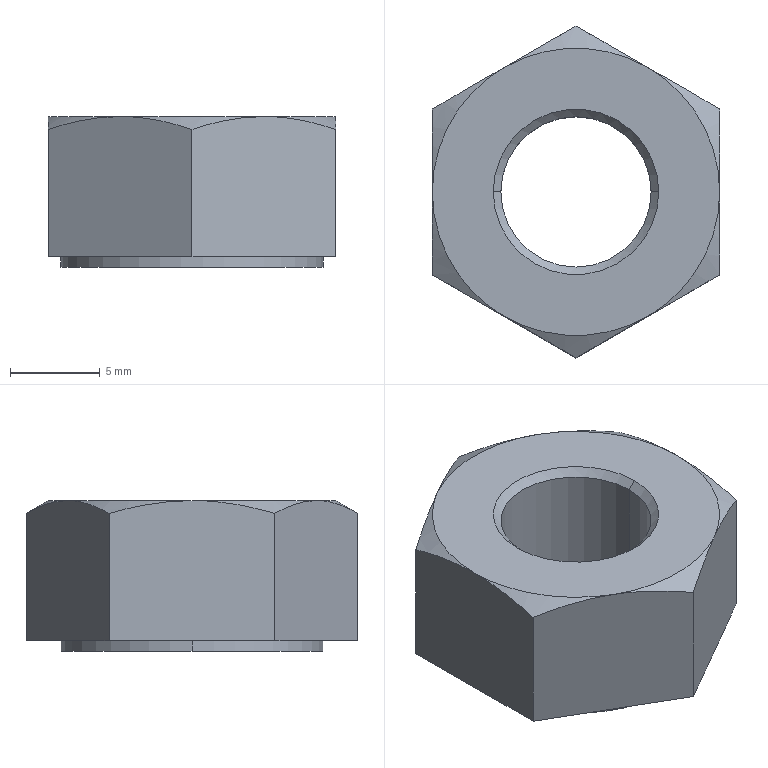Part | SolidWorks | features Cut 2, Chamfer 1, Extrusion 1 | 1 solid | 23 faces | box 16 x 18.475 x 8.4 mm | volume 1358 mm3 | cone 10 | plane 9 | cylinder 4 | commonest cylinder face diameters 8.376 x2 14.6 x2
STEP:
#1=CARTESIAN_POINT('',(-4.188,0.,7.98));
#2=VERTEX_POINT('',#1);
#3=CARTESIAN_POINT('',(4.188,0.,7.98));
#4=VERTEX_POINT('',#3);
#5=CARTESIAN_POINT('',(0.,0.,7.98));
#6=DIRECTION('',(0.,0.,1.));
#7=DIRECTION('',(1.,0.,0.));
#8=AXIS2_PLACEMENT_3D('',#5,#6,#7);
#9=CIRCLE('',#8,4.188);
#10=EDGE_CURVE('',#2,#4,#9,.T.);
#11=ORIENTED_EDGE('',*,*,#10,.F.);
#12=CARTESIAN_POINT('',(-4.608,0.,8.4));
#13=VERTEX_POINT('',#12);
#14=CARTESIAN_POINT('',(-4.188,0.,7.98));
#15=DIRECTION('',(-0.7071,0.,0.7071));
#16=VECTOR('',#15,1000.);
#17=LINE('',#14,#16);
#18=EDGE_CURVE('',#2,#13,#17,.T.);
#19=ORIENTED_EDGE('',*,*,#18,.T.);
#20=CARTESIAN_POINT('',(4.608,0.,8.4));
#21=VERTEX_POINT('',#20);
#22=CARTESIAN_POINT('',(0.,0.,8.4));
#23=DIRECTION('',(0.,0.,-1.));
#24=DIRECTION('',(1.,0.,0.));
#25=AXIS2_PLACEMENT_3D('',#22,#23,#24);
#26=CIRCLE('',#25,4.608);
#27=EDGE_CURVE('',#21,#13,#26,.T.);
#28=ORIENTED_EDGE('',*,*,#27,.F.);
#29=CARTESIAN_POINT('',(4.188,0.,7.98));
#30=DIRECTION('',(0.7071,0.,0.7071));
#31=VECTOR('',#30,1000.);
#32=LINE('',#29,#31);
#33=EDGE_CURVE('',#4,#21,#32,.T.);
#34=ORIENTED_EDGE('',*,*,#33,.F.);
#35=EDGE_LOOP('',(#11,#19,#28,#34));
#36=FACE_OUTER_BOUND('',#35,.T.);
#37=CARTESIAN_POINT('',(0.,0.,7.98));
#38=DIRECTION('',(0.,0.,1.));
#39=DIRECTION('',(1.,0.,0.));
#40=AXIS2_PLACEMENT_3D('',#37,#38,#39);
#41=CONICAL_SURFACE('',#40,4.188,0.7854);
#42=ADVANCED_FACE('',(#36),#41,.F.);
#43=CARTESIAN_POINT('',(4.188,0.,0.42));
#44=VERTEX_POINT('',#43);
#45=CARTESIAN_POINT('',(-4.188,0.,0.42));
#46=VERTEX_POINT('',#45);
#47=CARTESIAN_POINT('',(0.,0.,0.42));
#48=DIRECTION('',(0.,0.,-1.));
#49=DIRECTION('',(1.,0.,0.));
#50=AXIS2_PLACEMENT_3D('',#47,#48,#49);
#51=CIRCLE('',#50,4.188);
#52=EDGE_CURVE('',#44,#46,#51,.T.);
#53=ORIENTED_EDGE('',*,*,#52,.F.);
#54=CARTESIAN_POINT('',(4.608,0.,0.));
#55=VERTEX_POINT('',#54);
#56=CARTESIAN_POINT('',(4.608,0.,0.));
#57=DIRECTION('',(0.7071,0.,-0.7071));
#58=VECTOR('',#57,1000.);
#59=LINE('',#56,#58);
#60=EDGE_CURVE('',#44,#55,#59,.T.);
#61=ORIENTED_EDGE('',*,*,#60,.T.);
#62=CARTESIAN_POINT('',(-4.608,0.,0.));
#63=VERTEX_POINT('',#62);
#64=CARTESIAN_POINT('',(0.,0.,0.));
#65=DIRECTION('',(0.,0.,1.));
#66=DIRECTION('',(1.,0.,0.));
#67=AXIS2_PLACEMENT_3D('',#64,#65,#66);
#68=CIRCLE('',#67,4.608);
#69=EDGE_CURVE('',#63,#55,#68,.T.);
#70=ORIENTED_EDGE('',*,*,#69,.F.);
#71=CARTESIAN_POINT('',(-4.608,0.,0.));
#72=DIRECTION('',(-0.7071,0.,-0.7071));
#73=VECTOR('',#72,1000.);
#74=LINE('',#71,#73);
#75=EDGE_CURVE('',#46,#63,#74,.T.);
#76=ORIENTED_EDGE('',*,*,#75,.F.);
#77=EDGE_LOOP('',(#53,#61,#70,#76));
#78=FACE_OUTER_BOUND('',#77,.T.);
#79=CARTESIAN_POINT('',(0.,0.,0.));
#80=DIRECTION('',(0.,0.,-1.));
#81=DIRECTION('',(-1.,0.,0.));
#82=AXIS2_PLACEMENT_3D('',#79,#80,#81);
#83=CONICAL_SURFACE('',#82,4.608,0.7854);
#84=ADVANCED_FACE('',(#78),#83,.F.);
#85=CARTESIAN_POINT('',(7.3,0.,0.6));
#86=VERTEX_POINT('',#85);
#87=CARTESIAN_POINT('',(-7.3,0.,0.6));
#88=VERTEX_POINT('',#87);
#89=CARTESIAN_POINT('',(0.,0.,0.6));
#90=DIRECTION('',(0.,0.,1.));
#91=DIRECTION('',(1.,0.,0.));
#92=AXIS2_PLACEMENT_3D('',#89,#90,#91);
#93=CIRCLE('',#92,7.3);
#94=EDGE_CURVE('',#86,#88,#93,.T.);
#95=ORIENTED_EDGE('',*,*,#94,.F.);
#96=CARTESIAN_POINT('',(7.3,0.,0.));
#97=VERTEX_POINT('',#96);
#98=CARTESIAN_POINT('',(7.3,0.,0.6));
#99=DIRECTION('',(0.,0.,-1.));
#100=VECTOR('',#99,1000.);
#101=LINE('',#98,#100);
#102=EDGE_CURVE('',#86,#97,#101,.T.);
#103=ORIENTED_EDGE('',*,*,#102,.T.);
#104=CARTESIAN_POINT('',(-7.3,0.,0.));
#105=VERTEX_POINT('',#104);
#106=CARTESIAN_POINT('',(0.,0.,0.));
#107=DIRECTION('',(0.,0.,1.));
#108=DIRECTION('',(1.,0.,0.));
#109=AXIS2_PLACEMENT_3D('',#106,#107,#108);
#110=CIRCLE('',#109,7.3);
#111=EDGE_CURVE('',#97,#105,#110,.T.);
#112=ORIENTED_EDGE('',*,*,#111,.T.);
#113=CARTESIAN_POINT('',(-7.3,0.,0.6));
#114=DIRECTION('',(0.,0.,-1.));
#115=VECTOR('',#114,1000.);
#116=LINE('',#113,#115);
#117=EDGE_CURVE('',#88,#105,#116,.T.);
#118=ORIENTED_EDGE('',*,*,#117,.F.);
#119=EDGE_LOOP('',(#95,#103,#112,#118));
#120=FACE_OUTER_BOUND('',#119,.T.);
#121=CARTESIAN_POINT('',(0.,0.,0.6));
#122=DIRECTION('',(0.,0.,-1.));
#123=DIRECTION('',(-1.,0.,0.));
#124=AXIS2_PLACEMENT_3D('',#121,#122,#123);
#125=CYLINDRICAL_SURFACE('',#124,7.3);
#126=ADVANCED_FACE('',(#120),#125,.T.);
#127=ORIENTED_EDGE('',*,*,#10,.T.);
#128=CARTESIAN_POINT('',(4.188,0.,8.4));
#129=DIRECTION('',(0.,0.,-1.));
#130=VECTOR('',#129,1000.);
#131=LINE('',#128,#130);
#132=EDGE_CURVE('',#4,#44,#131,.T.);
#133=ORIENTED_EDGE('',*,*,#132,.T.);
#134=ORIENTED_EDGE('',*,*,#52,.T.);
#135=CARTESIAN_POINT('',(-4.188,0.,8.4));
#136=DIRECTION('',(0.,0.,-1.));
#137=VECTOR('',#136,1000.);
#138=LINE('',#135,#137);
#139=EDGE_CURVE('',#2,#46,#138,.T.);
#140=ORIENTED_EDGE('',*,*,#139,.F.);
#141=EDGE_LOOP('',(#127,#133,#134,#140));
#142=FACE_OUTER_BOUND('',#141,.T.);
#143=CARTESIAN_POINT('',(0.,0.,8.4));
#144=DIRECTION('',(0.,0.,-1.));
#145=DIRECTION('',(-1.,0.,0.));
#146=AXIS2_PLACEMENT_3D('',#143,#144,#145);
#147=CYLINDRICAL_SURFACE('',#146,4.188);
#148=ADVANCED_FACE('',(#142),#147,.F.);
#149=ORIENTED_EDGE('',*,*,#27,.T.);
#150=CARTESIAN_POINT('',(0.,0.,8.4));
#151=DIRECTION('',(0.,0.,-1.));
#152=DIRECTION('',(1.,0.,0.));
#153=AXIS2_PLACEMENT_3D('',#150,#151,#152);
#154=CIRCLE('',#153,4.608);
#155=EDGE_CURVE('',#13,#21,#154,.T.);
#156=ORIENTED_EDGE('',*,*,#155,.T.);
#157=EDGE_LOOP('',(#149,#156));
#158=FACE_BOUND('',#157,.T.);
#159=CARTESIAN_POINT('',(4.,-6.928,8.4));
#160=VERTEX_POINT('',#159);
#161=CARTESIAN_POINT('',(8.,0.,8.4));
#162=VERTEX_POINT('',#161);
#163=CARTESIAN_POINT('',(0.,0.,8.4));
#164=DIRECTION('',(0.,0.,1.));
#165=DIRECTION('',(1.,0.,0.));
#166=AXIS2_PLACEMENT_3D('',#163,#164,#165);
#167=CIRCLE('',#166,8.);
#168=EDGE_CURVE('',#160,#162,#167,.T.);
#169=ORIENTED_EDGE('',*,*,#168,.T.);
#170=CARTESIAN_POINT('',(4.,6.928,8.4));
#171=VERTEX_POINT('',#170);
#172=CARTESIAN_POINT('',(0.,0.,8.4));
#173=DIRECTION('',(0.,0.,1.));
#174=DIRECTION('',(1.,0.,0.));
#175=AXIS2_PLACEMENT_3D('',#172,#173,#174);
#176=CIRCLE('',#175,8.);
#177=EDGE_CURVE('',#162,#171,#176,.T.);
#178=ORIENTED_EDGE('',*,*,#177,.T.);
#179=CARTESIAN_POINT('',(-4.,6.928,8.4));
#180=VERTEX_POINT('',#179);
#181=CARTESIAN_POINT('',(0.,0.,8.4));
#182=DIRECTION('',(0.,0.,1.));
#183=DIRECTION('',(1.,0.,0.));
#184=AXIS2_PLACEMENT_3D('',#181,#182,#183);
#185=CIRCLE('',#184,8.);
#186=EDGE_CURVE('',#171,#180,#185,.T.);
#187=ORIENTED_EDGE('',*,*,#186,.T.);
#188=CARTESIAN_POINT('',(-8.,0.,8.4));
#189=VERTEX_POINT('',#188);
#190=CARTESIAN_POINT('',(0.,0.,8.4));
#191=DIRECTION('',(0.,0.,1.));
#192=DIRECTION('',(1.,0.,0.));
#193=AXIS2_PLACEMENT_3D('',#190,#191,#192);
#194=CIRCLE('',#193,8.);
#195=EDGE_CURVE('',#180,#189,#194,.T.);
#196=ORIENTED_EDGE('',*,*,#195,.T.);
#197=CARTESIAN_POINT('',(-4.,-6.928,8.4));
#198=VERTEX_POINT('',#197);
#199=CARTESIAN_POINT('',(0.,0.,8.4));
#200=DIRECTION('',(0.,0.,1.));
#201=DIRECTION('',(1.,0.,0.));
#202=AXIS2_PLACEMENT_3D('',#199,#200,#201);
#203=CIRCLE('',#202,8.);
#204=EDGE_CURVE('',#189,#198,#203,.T.);
#205=ORIENTED_EDGE('',*,*,#204,.T.);
#206=CARTESIAN_POINT('',(0.,0.,8.4));
#207=DIRECTION('',(0.,0.,1.));
#208=DIRECTION('',(1.,0.,0.));
#209=AXIS2_PLACEMENT_3D('',#206,#207,#208);
#210=CIRCLE('',#209,8.);
#211=EDGE_CURVE('',#198,#160,#210,.T.);
#212=ORIENTED_EDGE('',*,*,#211,.T.);
#213=EDGE_LOOP('',(#169,#178,#187,#196,#205,#212));
#214=FACE_OUTER_BOUND('',#213,.T.);
#215=CARTESIAN_POINT('',(-8.,13.856,8.4));
#216=DIRECTION('',(0.,0.,1.));
#217=DIRECTION('',(1.,0.,0.));
#218=AXIS2_PLACEMENT_3D('',#215,#216,#217);
#219=PLANE('',#218);
#220=ADVANCED_FACE('',(#158,#214),#219,.T.);
#221=CARTESIAN_POINT('',(8.,4.619,7.685));
#222=VERTEX_POINT('',#221);
#223=CARTESIAN_POINT('',(8.,4.619,7.685));
#224=CARTESIAN_POINT('',(7.346,4.997,7.904));
#225=CARTESIAN_POINT('',(6.687,5.377,8.083));
#226=CARTESIAN_POINT('',(5.354,6.146,8.332));
#227=CARTESIAN_POINT('',(4.681,6.535,8.4));
#228=CARTESIAN_POINT('',(4.,6.928,8.4));
#229=B_SPLINE_CURVE_WITH_KNOTS('',3,(#223,#224,#225,#226,#227,#228),.UNSPECIFIED.,.F.,.F.,(4,2,4),(0.000000238,0.002337,0.004674),.UNSPECIFIED.);
#230=EDGE_CURVE('',#222,#171,#229,.T.);
#231=ORIENTED_EDGE('',*,*,#230,.F.);
#232=CARTESIAN_POINT('',(8.,4.619,0.6));
#233=VERTEX_POINT('',#232);
#234=CARTESIAN_POINT('',(8.,4.619,8.4));
#235=DIRECTION('',(0.,0.,-1.));
#236=VECTOR('',#235,1000.);
#237=LINE('',#234,#236);
#238=EDGE_CURVE('',#222,#233,#237,.T.);
#239=ORIENTED_EDGE('',*,*,#238,.T.);
#240=CARTESIAN_POINT('',(0.,9.238,0.6));
#241=VERTEX_POINT('',#240);
#242=CARTESIAN_POINT('',(8.,4.619,0.6));
#243=DIRECTION('',(-0.866,0.5,0.));
#244=VECTOR('',#243,1000.);
#245=LINE('',#242,#244);
#246=EDGE_CURVE('',#233,#241,#245,.T.);
#247=ORIENTED_EDGE('',*,*,#246,.T.);
#248=CARTESIAN_POINT('',(0.,9.238,7.685));
#249=VERTEX_POINT('',#248);
#250=CARTESIAN_POINT('',(0.,9.238,8.4));
#251=DIRECTION('',(0.,0.,-1.));
#252=VECTOR('',#251,1000.);
#253=LINE('',#250,#252);
#254=EDGE_CURVE('',#249,#241,#253,.T.);
#255=ORIENTED_EDGE('',*,*,#254,.F.);
#256=CARTESIAN_POINT('',(4.,6.928,8.4));
#257=CARTESIAN_POINT('',(3.661,7.124,8.4));
#258=CARTESIAN_POINT('',(3.32,7.321,8.383));
#259=CARTESIAN_POINT('',(2.645,7.711,8.318));
#260=CARTESIAN_POINT('',(2.31,7.904,8.269));
#261=CARTESIAN_POINT('',(1.311,8.481,8.083));
#262=CARTESIAN_POINT('',(0.6527,8.861,7.903));
#263=CARTESIAN_POINT('',(0.,9.238,7.685));
#264=B_SPLINE_CURVE_WITH_KNOTS('',3,(#256,#257,#258,#259,#260,#261,#262,#263),.UNSPECIFIED.,.F.,.F.,(4,2,2,4),(0.004674,0.005838,0.007002,0.00933),.UNSPECIFIED.);
#265=EDGE_CURVE('',#171,#249,#264,.T.);
#266=ORIENTED_EDGE('',*,*,#265,.F.);
#267=EDGE_LOOP('',(#231,#239,#247,#255,#266));
#268=FACE_OUTER_BOUND('',#267,.T.);
#269=CARTESIAN_POINT('',(8.,4.619,8.4));
#270=DIRECTION('',(-0.5,-0.866,0.));
#271=DIRECTION('',(0.866,-0.5,0.));
#272=AXIS2_PLACEMENT_3D('',#269,#270,#271);
#273=PLANE('',#272);
#274=ADVANCED_FACE('',(#268),#273,.F.);
#275=CARTESIAN_POINT('',(0.,9.238,7.685));
#276=CARTESIAN_POINT('',(-0.6543,8.86,7.904));
#277=CARTESIAN_POINT('',(-1.313,8.479,8.083));
#278=CARTESIAN_POINT('',(-2.646,7.71,8.332));
#279=CARTESIAN_POINT('',(-3.319,7.322,8.4));
#280=CARTESIAN_POINT('',(-4.,6.928,8.4));
#281=B_SPLINE_CURVE_WITH_KNOTS('',3,(#275,#276,#277,#278,#279,#280),.UNSPECIFIED.,.F.,.F.,(4,2,4),(0.000000238,0.002337,0.004674),.UNSPECIFIED.);
#282=EDGE_CURVE('',#249,#180,#281,.T.);
#283=ORIENTED_EDGE('',*,*,#282,.F.);
#284=ORIENTED_EDGE('',*,*,#254,.T.);
#285=CARTESIAN_POINT('',(-8.,4.619,0.6));
#286=VERTEX_POINT('',#285);
#287=CARTESIAN_POINT('',(0.,9.238,0.6));
#288=DIRECTION('',(-0.866,-0.5,0.));
#289=VECTOR('',#288,1000.);
#290=LINE('',#287,#289);
#291=EDGE_CURVE('',#241,#286,#290,.T.);
#292=ORIENTED_EDGE('',*,*,#291,.T.);
#293=CARTESIAN_POINT('',(-8.,4.619,7.685));
#294=VERTEX_POINT('',#293);
#295=CARTESIAN_POINT('',(-8.,4.619,8.4));
#296=DIRECTION('',(0.,0.,-1.));
#297=VECTOR('',#296,1000.);
#298=LINE('',#295,#297);
#299=EDGE_CURVE('',#294,#286,#298,.T.);
#300=ORIENTED_EDGE('',*,*,#299,.F.);
#301=CARTESIAN_POINT('',(-4.,6.928,8.4));
#302=CARTESIAN_POINT('',(-4.339,6.732,8.4));
#303=CARTESIAN_POINT('',(-4.68,6.535,8.383));
#304=CARTESIAN_POINT('',(-5.355,6.146,8.318));
#305=CARTESIAN_POINT('',(-5.69,5.952,8.269));
#306=CARTESIAN_POINT('',(-6.689,5.376,8.083));
#307=CARTESIAN_POINT('',(-7.347,4.996,7.903));
#308=CARTESIAN_POINT('',(-8.,4.619,7.685));
#309=B_SPLINE_CURVE_WITH_KNOTS('',3,(#301,#302,#303,#304,#305,#306,#307,#308),.UNSPECIFIED.,.F.,.F.,(4,2,2,4),(0.004674,0.005838,0.007002,0.00933),.UNSPECIFIED.);
#310=EDGE_CURVE('',#180,#294,#309,.T.);
#311=ORIENTED_EDGE('',*,*,#310,.F.);
#312=EDGE_LOOP('',(#283,#284,#292,#300,#311));
#313=FACE_OUTER_BOUND('',#312,.T.);
#314=CARTESIAN_POINT('',(0.,9.238,8.4));
#315=DIRECTION('',(0.5,-0.866,0.));
#316=DIRECTION('',(0.866,0.5,0.));
#317=AXIS2_PLACEMENT_3D('',#314,#315,#316);
#318=PLANE('',#317);
#319=ADVANCED_FACE('',(#313),#318,.F.);
#320=CARTESIAN_POINT('',(-8.,4.619,7.685));
#321=CARTESIAN_POINT('',(-8.,3.872,7.901));
#322=CARTESIAN_POINT('',(-8.,3.115,8.081));
#323=CARTESIAN_POINT('',(-8.,1.573,8.331));
#324=CARTESIAN_POINT('',(-8.,0.7816,8.4));
#325=CARTESIAN_POINT('',(-8.,0.,8.4));
#326=B_SPLINE_CURVE_WITH_KNOTS('',3,(#320,#321,#322,#323,#324,#325),.UNSPECIFIED.,.F.,.F.,(4,2,4),(0.02573,0.02807,0.03041),.UNSPECIFIED.);
#327=EDGE_CURVE('',#294,#189,#326,.T.);
#328=ORIENTED_EDGE('',*,*,#327,.F.);
#329=ORIENTED_EDGE('',*,*,#299,.T.);
#330=CARTESIAN_POINT('',(-8.,-4.619,0.6));
#331=VERTEX_POINT('',#330);
#332=CARTESIAN_POINT('',(-8.,4.619,0.6));
#333=DIRECTION('',(0.,-1.,0.));
#334=VECTOR('',#333,1000.);
#335=LINE('',#332,#334);
#336=EDGE_CURVE('',#286,#331,#335,.T.);
#337=ORIENTED_EDGE('',*,*,#336,.T.);
#338=CARTESIAN_POINT('',(-8.,-4.619,7.685));
#339=VERTEX_POINT('',#338);
#340=CARTESIAN_POINT('',(-8.,-4.619,8.4));
#341=DIRECTION('',(0.,0.,-1.));
#342=VECTOR('',#341,1000.);
#343=LINE('',#340,#342);
#344=EDGE_CURVE('',#339,#331,#343,.T.);
#345=ORIENTED_EDGE('',*,*,#344,.F.);
#346=CARTESIAN_POINT('',(-8.,0.,8.4));
#347=CARTESIAN_POINT('',(-8.,-0.781,8.4));
#348=CARTESIAN_POINT('',(-8.,-1.556,8.333));
#349=CARTESIAN_POINT('',(-8.,-3.098,8.084));
#350=CARTESIAN_POINT('',(-8.,-3.867,7.902));
#351=CARTESIAN_POINT('',(-8.,-4.619,7.685));
#352=B_SPLINE_CURVE_WITH_KNOTS('',3,(#346,#347,#348,#349,#350,#351),.UNSPECIFIED.,.F.,.F.,(4,2,4),(0.03041,0.03275,0.03509),.UNSPECIFIED.);
#353=EDGE_CURVE('',#189,#339,#352,.T.);
#354=ORIENTED_EDGE('',*,*,#353,.F.);
#355=EDGE_LOOP('',(#328,#329,#337,#345,#354));
#356=FACE_OUTER_BOUND('',#355,.T.);
#357=CARTESIAN_POINT('',(-8.,4.619,8.4));
#358=DIRECTION('',(1.,0.,0.));
#359=DIRECTION('',(0.,1.,0.));
#360=AXIS2_PLACEMENT_3D('',#357,#358,#359);
#361=PLANE('',#360);
#362=ADVANCED_FACE('',(#356),#361,.F.);
#363=CARTESIAN_POINT('',(-8.,-4.619,7.685));
#364=CARTESIAN_POINT('',(-7.346,-4.997,7.904));
#365=CARTESIAN_POINT('',(-6.687,-5.377,8.083));
#366=CARTESIAN_POINT('',(-5.354,-6.146,8.332));
#367=CARTESIAN_POINT('',(-4.681,-6.535,8.4));
#368=CARTESIAN_POINT('',(-4.,-6.928,8.4));
#369=B_SPLINE_CURVE_WITH_KNOTS('',3,(#363,#364,#365,#366,#367,#368),.UNSPECIFIED.,.F.,.F.,(4,2,4),(0.000000238,0.002337,0.004674),.UNSPECIFIED.);
#370=EDGE_CURVE('',#339,#198,#369,.T.);
#371=ORIENTED_EDGE('',*,*,#370,.F.);
#372=ORIENTED_EDGE('',*,*,#344,.T.);
#373=CARTESIAN_POINT('',(0.,-9.238,0.6));
#374=VERTEX_POINT('',#373);
#375=CARTESIAN_POINT('',(-8.,-4.619,0.6));
#376=DIRECTION('',(0.866,-0.5,0.));
#377=VECTOR('',#376,1000.);
#378=LINE('',#375,#377);
#379=EDGE_CURVE('',#331,#374,#378,.T.);
#380=ORIENTED_EDGE('',*,*,#379,.T.);
#381=CARTESIAN_POINT('',(0.,-9.238,7.685));
#382=VERTEX_POINT('',#381);
#383=CARTESIAN_POINT('',(0.,-9.238,8.4));
#384=DIRECTION('',(0.,0.,-1.));
#385=VECTOR('',#384,1000.);
#386=LINE('',#383,#385);
#387=EDGE_CURVE('',#382,#374,#386,.T.);
#388=ORIENTED_EDGE('',*,*,#387,.F.);
#389=CARTESIAN_POINT('',(-4.,-6.928,8.4));
#390=CARTESIAN_POINT('',(-3.661,-7.124,8.4));
#391=CARTESIAN_POINT('',(-3.32,-7.321,8.383));
#392=CARTESIAN_POINT('',(-2.645,-7.711,8.318));
#393=CARTESIAN_POINT('',(-2.31,-7.904,8.269));
#394=CARTESIAN_POINT('',(-1.311,-8.481,8.083));
#395=CARTESIAN_POINT('',(-0.6527,-8.861,7.903));
#396=CARTESIAN_POINT('',(0.,-9.238,7.685));
#397=B_SPLINE_CURVE_WITH_KNOTS('',3,(#389,#390,#391,#392,#393,#394,#395,#396),.UNSPECIFIED.,.F.,.F.,(4,2,2,4),(0.004674,0.005838,0.007002,0.00933),.UNSPECIFIED.);
#398=EDGE_CURVE('',#198,#382,#397,.T.);
#399=ORIENTED_EDGE('',*,*,#398,.F.);
#400=EDGE_LOOP('',(#371,#372,#380,#388,#399));
#401=FACE_OUTER_BOUND('',#400,.T.);
#402=CARTESIAN_POINT('',(-8.,-4.619,8.4));
#403=DIRECTION('',(0.5,0.866,0.));
#404=DIRECTION('',(-0.866,0.5,0.));
#405=AXIS2_PLACEMENT_3D('',#402,#403,#404);
#406=PLANE('',#405);
#407=ADVANCED_FACE('',(#401),#406,.F.);
#408=CARTESIAN_POINT('',(0.,-9.238,7.685));
#409=CARTESIAN_POINT('',(0.6543,-8.86,7.904));
#410=CARTESIAN_POINT('',(1.313,-8.479,8.083));
#411=CARTESIAN_POINT('',(2.646,-7.71,8.332));
#412=CARTESIAN_POINT('',(3.319,-7.322,8.4));
#413=CARTESIAN_POINT('',(4.,-6.928,8.4));
#414=B_SPLINE_CURVE_WITH_KNOTS('',3,(#408,#409,#410,#411,#412,#413),.UNSPECIFIED.,.F.,.F.,(4,2,4),(0.000000238,0.002337,0.004674),.UNSPECIFIED.);
#415=EDGE_CURVE('',#382,#160,#414,.T.);
#416=ORIENTED_EDGE('',*,*,#415,.F.);
#417=ORIENTED_EDGE('',*,*,#387,.T.);
#418=CARTESIAN_POINT('',(8.,-4.619,0.6));
#419=VERTEX_POINT('',#418);
#420=CARTESIAN_POINT('',(0.,-9.238,0.6));
#421=DIRECTION('',(0.866,0.5,0.));
#422=VECTOR('',#421,1000.);
#423=LINE('',#420,#422);
#424=EDGE_CURVE('',#374,#419,#423,.T.);
#425=ORIENTED_EDGE('',*,*,#424,.T.);
#426=CARTESIAN_POINT('',(8.,-4.619,7.685));
#427=VERTEX_POINT('',#426);
#428=CARTESIAN_POINT('',(8.,-4.619,8.4));
#429=DIRECTION('',(0.,0.,-1.));
#430=VECTOR('',#429,1000.);
#431=LINE('',#428,#430);
#432=EDGE_CURVE('',#427,#419,#431,.T.);
#433=ORIENTED_EDGE('',*,*,#432,.F.);
#434=CARTESIAN_POINT('',(4.,-6.928,8.4));
#435=CARTESIAN_POINT('',(4.339,-6.732,8.4));
#436=CARTESIAN_POINT('',(4.68,-6.535,8.383));
#437=CARTESIAN_POINT('',(5.355,-6.146,8.318));
#438=CARTESIAN_POINT('',(5.69,-5.952,8.269));
#439=CARTESIAN_POINT('',(6.689,-5.376,8.083));
#440=CARTESIAN_POINT('',(7.347,-4.996,7.903));
#441=CARTESIAN_POINT('',(8.,-4.619,7.685));
#442=B_SPLINE_CURVE_WITH_KNOTS('',3,(#434,#435,#436,#437,#438,#439,#440,#441),.UNSPECIFIED.,.F.,.F.,(4,2,2,4),(0.004674,0.005838,0.007002,0.00933),.UNSPECIFIED.);
#443=EDGE_CURVE('',#160,#427,#442,.T.);
#444=ORIENTED_EDGE('',*,*,#443,.F.);
#445=EDGE_LOOP('',(#416,#417,#425,#433,#444));
#446=FACE_OUTER_BOUND('',#445,.T.);
#447=CARTESIAN_POINT('',(0.,-9.238,8.4));
#448=DIRECTION('',(-0.5,0.866,0.));
#449=DIRECTION('',(-0.866,-0.5,0.));
#450=AXIS2_PLACEMENT_3D('',#447,#448,#449);
#451=PLANE('',#450);
#452=ADVANCED_FACE('',(#446),#451,.F.);
#453=CARTESIAN_POINT('',(8.,-4.619,7.685));
#454=CARTESIAN_POINT('',(8.,-3.867,7.902));
#455=CARTESIAN_POINT('',(8.,-3.098,8.084));
#456=CARTESIAN_POINT('',(8.,-1.556,8.333));
#457=CARTESIAN_POINT('',(8.,-0.781,8.4));
#458=CARTESIAN_POINT('',(8.,0.,8.4));
#459=B_SPLINE_CURVE_WITH_KNOTS('',3,(#453,#454,#455,#456,#457,#458),.UNSPECIFIED.,.F.,.F.,(4,2,4),(0.008427,0.01076,0.0131),.UNSPECIFIED.);
#460=EDGE_CURVE('',#427,#162,#459,.T.);
#461=ORIENTED_EDGE('',*,*,#460,.F.);
#462=ORIENTED_EDGE('',*,*,#432,.T.);
#463=CARTESIAN_POINT('',(8.,-4.619,0.6));
#464=DIRECTION('',(0.,1.,0.));
#465=VECTOR('',#464,1000.);
#466=LINE('',#463,#465);
#467=EDGE_CURVE('',#419,#233,#466,.T.);
#468=ORIENTED_EDGE('',*,*,#467,.T.);
#469=ORIENTED_EDGE('',*,*,#238,.F.);
#470=CARTESIAN_POINT('',(8.,0.,8.4));
#471=CARTESIAN_POINT('',(8.,0.7816,8.4));
#472=CARTESIAN_POINT('',(8.,1.573,8.331));
#473=CARTESIAN_POINT('',(8.,3.115,8.081));
#474=CARTESIAN_POINT('',(8.,3.872,7.901));
#475=CARTESIAN_POINT('',(8.,4.619,7.685));
#476=B_SPLINE_CURVE_WITH_KNOTS('',3,(#470,#471,#472,#473,#474,#475),.UNSPECIFIED.,.F.,.F.,(4,2,4),(0.0131,0.01544,0.01778),.UNSPECIFIED.);
#477=EDGE_CURVE('',#162,#222,#476,.T.);
#478=ORIENTED_EDGE('',*,*,#477,.F.);
#479=EDGE_LOOP('',(#461,#462,#468,#469,#478));
#480=FACE_OUTER_BOUND('',#479,.T.);
#481=CARTESIAN_POINT('',(8.,-4.619,8.4));
#482=DIRECTION('',(-1.,0.,0.));
#483=DIRECTION('',(0.,0.,1.));
#484=AXIS2_PLACEMENT_3D('',#481,#482,#483);
#485=PLANE('',#484);
#486=ADVANCED_FACE('',(#480),#485,.F.);
#487=ORIENTED_EDGE('',*,*,#69,.T.);
#488=CARTESIAN_POINT('',(0.,0.,0.));
#489=DIRECTION('',(0.,0.,1.));
#490=DIRECTION('',(1.,0.,0.));
#491=AXIS2_PLACEMENT_3D('',#488,#489,#490);
#492=CIRCLE('',#491,4.608);
#493=EDGE_CURVE('',#55,#63,#492,.T.);
#494=ORIENTED_EDGE('',*,*,#493,.T.);
#495=EDGE_LOOP('',(#487,#494));
#496=FACE_BOUND('',#495,.T.);
#497=CARTESIAN_POINT('',(0.,0.,0.));
#498=DIRECTION('',(0.,0.,1.));
#499=DIRECTION('',(1.,0.,0.));
#500=AXIS2_PLACEMENT_3D('',#497,#498,#499);
#501=CIRCLE('',#500,7.3);
#502=EDGE_CURVE('',#105,#97,#501,.T.);
#503=ORIENTED_EDGE('',*,*,#502,.F.);
#504=ORIENTED_EDGE('',*,*,#111,.F.);
#505=EDGE_LOOP('',(#503,#504));
#506=FACE_OUTER_BOUND('',#505,.T.);
#507=CARTESIAN_POINT('',(-8.,13.856,0.));
#508=DIRECTION('',(0.,0.,1.));
#509=DIRECTION('',(1.,0.,0.));
#510=AXIS2_PLACEMENT_3D('',#507,#508,#509);
#511=PLANE('',#510);
#512=ADVANCED_FACE('',(#496,#506),#511,.F.);
#513=ORIENTED_EDGE('',*,*,#132,.F.);
#514=CARTESIAN_POINT('',(0.,0.,7.98));
#515=DIRECTION('',(0.,0.,1.));
#516=DIRECTION('',(1.,0.,0.));
#517=AXIS2_PLACEMENT_3D('',#514,#515,#516);
#518=CIRCLE('',#517,4.188);
#519=EDGE_CURVE('',#4,#2,#518,.T.);
#520=ORIENTED_EDGE('',*,*,#519,.T.);
#521=ORIENTED_EDGE('',*,*,#139,.T.);
#522=CARTESIAN_POINT('',(0.,0.,0.42));
#523=DIRECTION('',(0.,0.,-1.));
#524=DIRECTION('',(1.,0.,0.));
#525=AXIS2_PLACEMENT_3D('',#522,#523,#524);
#526=CIRCLE('',#525,4.188);
#527=EDGE_CURVE('',#46,#44,#526,.T.);
#528=ORIENTED_EDGE('',*,*,#527,.T.);
#529=EDGE_LOOP('',(#513,#520,#521,#528));
#530=FACE_OUTER_BOUND('',#529,.T.);
#531=CARTESIAN_POINT('',(0.,0.,8.4));
#532=DIRECTION('',(0.,0.,-1.));
#533=DIRECTION('',(-1.,0.,0.));
#534=AXIS2_PLACEMENT_3D('',#531,#532,#533);
#535=CYLINDRICAL_SURFACE('',#534,4.188);
#536=ADVANCED_FACE('',(#530),#535,.F.);
#537=CARTESIAN_POINT('',(0.,0.,0.6));
#538=DIRECTION('',(0.,0.,1.));
#539=DIRECTION('',(1.,0.,0.));
#540=AXIS2_PLACEMENT_3D('',#537,#538,#539);
#541=CIRCLE('',#540,7.3);
#542=EDGE_CURVE('',#88,#86,#541,.T.);
#543=ORIENTED_EDGE('',*,*,#542,.T.);
#544=ORIENTED_EDGE('',*,*,#94,.T.);
#545=EDGE_LOOP('',(#543,#544));
#546=FACE_BOUND('',#545,.T.);
#547=ORIENTED_EDGE('',*,*,#467,.F.);
#548=ORIENTED_EDGE('',*,*,#424,.F.);
#549=ORIENTED_EDGE('',*,*,#379,.F.);
#550=ORIENTED_EDGE('',*,*,#336,.F.);
#551=ORIENTED_EDGE('',*,*,#291,.F.);
#552=ORIENTED_EDGE('',*,*,#246,.F.);
#553=EDGE_LOOP('',(#547,#548,#549,#550,#551,#552));
#554=FACE_OUTER_BOUND('',#553,.T.);
#555=CARTESIAN_POINT('',(0.,0.,0.6));
#556=DIRECTION('',(0.,0.,1.));
#557=DIRECTION('',(1.,0.,0.));
#558=AXIS2_PLACEMENT_3D('',#555,#556,#557);
#559=PLANE('',#558);
#560=ADVANCED_FACE('',(#546,#554),#559,.F.);
#561=ORIENTED_EDGE('',*,*,#102,.F.);
#562=ORIENTED_EDGE('',*,*,#542,.F.);
#563=ORIENTED_EDGE('',*,*,#117,.T.);
#564=ORIENTED_EDGE('',*,*,#502,.T.);
#565=EDGE_LOOP('',(#561,#562,#563,#564));
#566=FACE_OUTER_BOUND('',#565,.T.);
#567=CARTESIAN_POINT('',(0.,0.,0.6));
#568=DIRECTION('',(0.,0.,-1.));
#569=DIRECTION('',(-1.,0.,0.));
#570=AXIS2_PLACEMENT_3D('',#567,#568,#569);
#571=CYLINDRICAL_SURFACE('',#570,7.3);
#572=ADVANCED_FACE('',(#566),#571,.T.);
#573=ORIENTED_EDGE('',*,*,#230,.T.);
#574=ORIENTED_EDGE('',*,*,#177,.F.);
#575=ORIENTED_EDGE('',*,*,#477,.T.);
#576=EDGE_LOOP('',(#573,#574,#575));
#577=FACE_OUTER_BOUND('',#576,.T.);
#578=CARTESIAN_POINT('',(0.,0.,8.4));
#579=DIRECTION('',(0.,0.,-1.));
#580=DIRECTION('',(1.,0.,0.));
#581=AXIS2_PLACEMENT_3D('',#578,#579,#580);
#582=CONICAL_SURFACE('',#581,8.,1.047);
#583=ADVANCED_FACE('',(#577),#582,.T.);
#584=ORIENTED_EDGE('',*,*,#443,.T.);
#585=ORIENTED_EDGE('',*,*,#460,.T.);
#586=ORIENTED_EDGE('',*,*,#168,.F.);
#587=EDGE_LOOP('',(#584,#585,#586));
#588=FACE_OUTER_BOUND('',#587,.T.);
#589=CARTESIAN_POINT('',(0.,0.,8.4));
#590=DIRECTION('',(0.,0.,-1.));
#591=DIRECTION('',(1.,0.,0.));
#592=AXIS2_PLACEMENT_3D('',#589,#590,#591);
#593=CONICAL_SURFACE('',#592,8.,1.047);
#594=ADVANCED_FACE('',(#588),#593,.T.);
#595=ORIENTED_EDGE('',*,*,#398,.T.);
#596=ORIENTED_EDGE('',*,*,#415,.T.);
#597=ORIENTED_EDGE('',*,*,#211,.F.);
#598=EDGE_LOOP('',(#595,#596,#597));
#599=FACE_OUTER_BOUND('',#598,.T.);
#600=CARTESIAN_POINT('',(0.,0.,8.4));
#601=DIRECTION('',(0.,0.,-1.));
#602=DIRECTION('',(1.,0.,0.));
#603=AXIS2_PLACEMENT_3D('',#600,#601,#602);
#604=CONICAL_SURFACE('',#603,8.,1.047);
#605=ADVANCED_FACE('',(#599),#604,.T.);
#606=ORIENTED_EDGE('',*,*,#353,.T.);
#607=ORIENTED_EDGE('',*,*,#370,.T.);
#608=ORIENTED_EDGE('',*,*,#204,.F.);
#609=EDGE_LOOP('',(#606,#607,#608));
#610=FACE_OUTER_BOUND('',#609,.T.);
#611=CARTESIAN_POINT('',(0.,0.,8.4));
#612=DIRECTION('',(0.,0.,-1.));
#613=DIRECTION('',(1.,0.,0.));
#614=AXIS2_PLACEMENT_3D('',#611,#612,#613);
#615=CONICAL_SURFACE('',#614,8.,1.047);
#616=ADVANCED_FACE('',(#610),#615,.T.);
#617=ORIENTED_EDGE('',*,*,#310,.T.);
#618=ORIENTED_EDGE('',*,*,#327,.T.);
#619=ORIENTED_EDGE('',*,*,#195,.F.);
#620=EDGE_LOOP('',(#617,#618,#619));
#621=FACE_OUTER_BOUND('',#620,.T.);
#622=CARTESIAN_POINT('',(0.,0.,8.4));
#623=DIRECTION('',(0.,0.,-1.));
#624=DIRECTION('',(1.,0.,0.));
#625=AXIS2_PLACEMENT_3D('',#622,#623,#624);
#626=CONICAL_SURFACE('',#625,8.,1.047);
#627=ADVANCED_FACE('',(#621),#626,.T.);
#628=ORIENTED_EDGE('',*,*,#265,.T.);
#629=ORIENTED_EDGE('',*,*,#282,.T.);
#630=ORIENTED_EDGE('',*,*,#186,.F.);
#631=EDGE_LOOP('',(#628,#629,#630));
#632=FACE_OUTER_BOUND('',#631,.T.);
#633=CARTESIAN_POINT('',(0.,0.,8.4));
#634=DIRECTION('',(0.,0.,-1.));
#635=DIRECTION('',(1.,0.,0.));
#636=AXIS2_PLACEMENT_3D('',#633,#634,#635);
#637=CONICAL_SURFACE('',#636,8.,1.047);
#638=ADVANCED_FACE('',(#632),#637,.T.);
#639=ORIENTED_EDGE('',*,*,#60,.F.);
#640=ORIENTED_EDGE('',*,*,#527,.F.);
#641=ORIENTED_EDGE('',*,*,#75,.T.);
#642=ORIENTED_EDGE('',*,*,#493,.F.);
#643=EDGE_LOOP('',(#639,#640,#641,#642));
#644=FACE_OUTER_BOUND('',#643,.T.);
#645=CARTESIAN_POINT('',(0.,0.,0.));
#646=DIRECTION('',(0.,0.,-1.));
#647=DIRECTION('',(-1.,0.,0.));
#648=AXIS2_PLACEMENT_3D('',#645,#646,#647);
#649=CONICAL_SURFACE('',#648,4.608,0.7854);
#650=ADVANCED_FACE('',(#644),#649,.F.);
#651=ORIENTED_EDGE('',*,*,#18,.F.);
#652=ORIENTED_EDGE('',*,*,#519,.F.);
#653=ORIENTED_EDGE('',*,*,#33,.T.);
#654=ORIENTED_EDGE('',*,*,#155,.F.);
#655=EDGE_LOOP('',(#651,#652,#653,#654));
#656=FACE_OUTER_BOUND('',#655,.T.);
#657=CARTESIAN_POINT('',(0.,0.,7.98));
#658=DIRECTION('',(0.,0.,1.));
#659=DIRECTION('',(1.,0.,0.));
#660=AXIS2_PLACEMENT_3D('',#657,#658,#659);
#661=CONICAL_SURFACE('',#660,4.188,0.7854);
#662=ADVANCED_FACE('',(#656),#661,.F.);
#663=CLOSED_SHELL('',(#42,#84,#126,#148,#220,#274,#319,#362,#407,#452,#486,#512,#536,#560,#572,#583,#594,#605,#616,#627,#638,#650,#662));
#664=MANIFOLD_SOLID_BREP('',#663);
#665=CARTESIAN_POINT('',(0.,0.,0.));
#666=DIRECTION('',(0.,0.,1.));
#667=DIRECTION('',(1.,0.,0.));
#668=AXIS2_PLACEMENT_3D('',#665,#666,#667);
#669=(LENGTH_UNIT()NAMED_UNIT(*)SI_UNIT(.MILLI.,.METRE.));
#670=UNCERTAINTY_MEASURE_WITH_UNIT(LENGTH_MEASURE(0.00001),#669,'','');
#671=(NAMED_UNIT(*)PLANE_ANGLE_UNIT()SI_UNIT($,.RADIAN.));
#672=(NAMED_UNIT(*)SI_UNIT($,.STERADIAN.)SOLID_ANGLE_UNIT());
#673=(GEOMETRIC_REPRESENTATION_CONTEXT(3)GLOBAL_UNCERTAINTY_ASSIGNED_CONTEXT((#670))GLOBAL_UNIT_ASSIGNED_CONTEXT((#669,#671,#672))REPRESENTATION_CONTEXT('',''));
#674=ADVANCED_BREP_SHAPE_REPRESENTATION('',(#664,#668),#673);